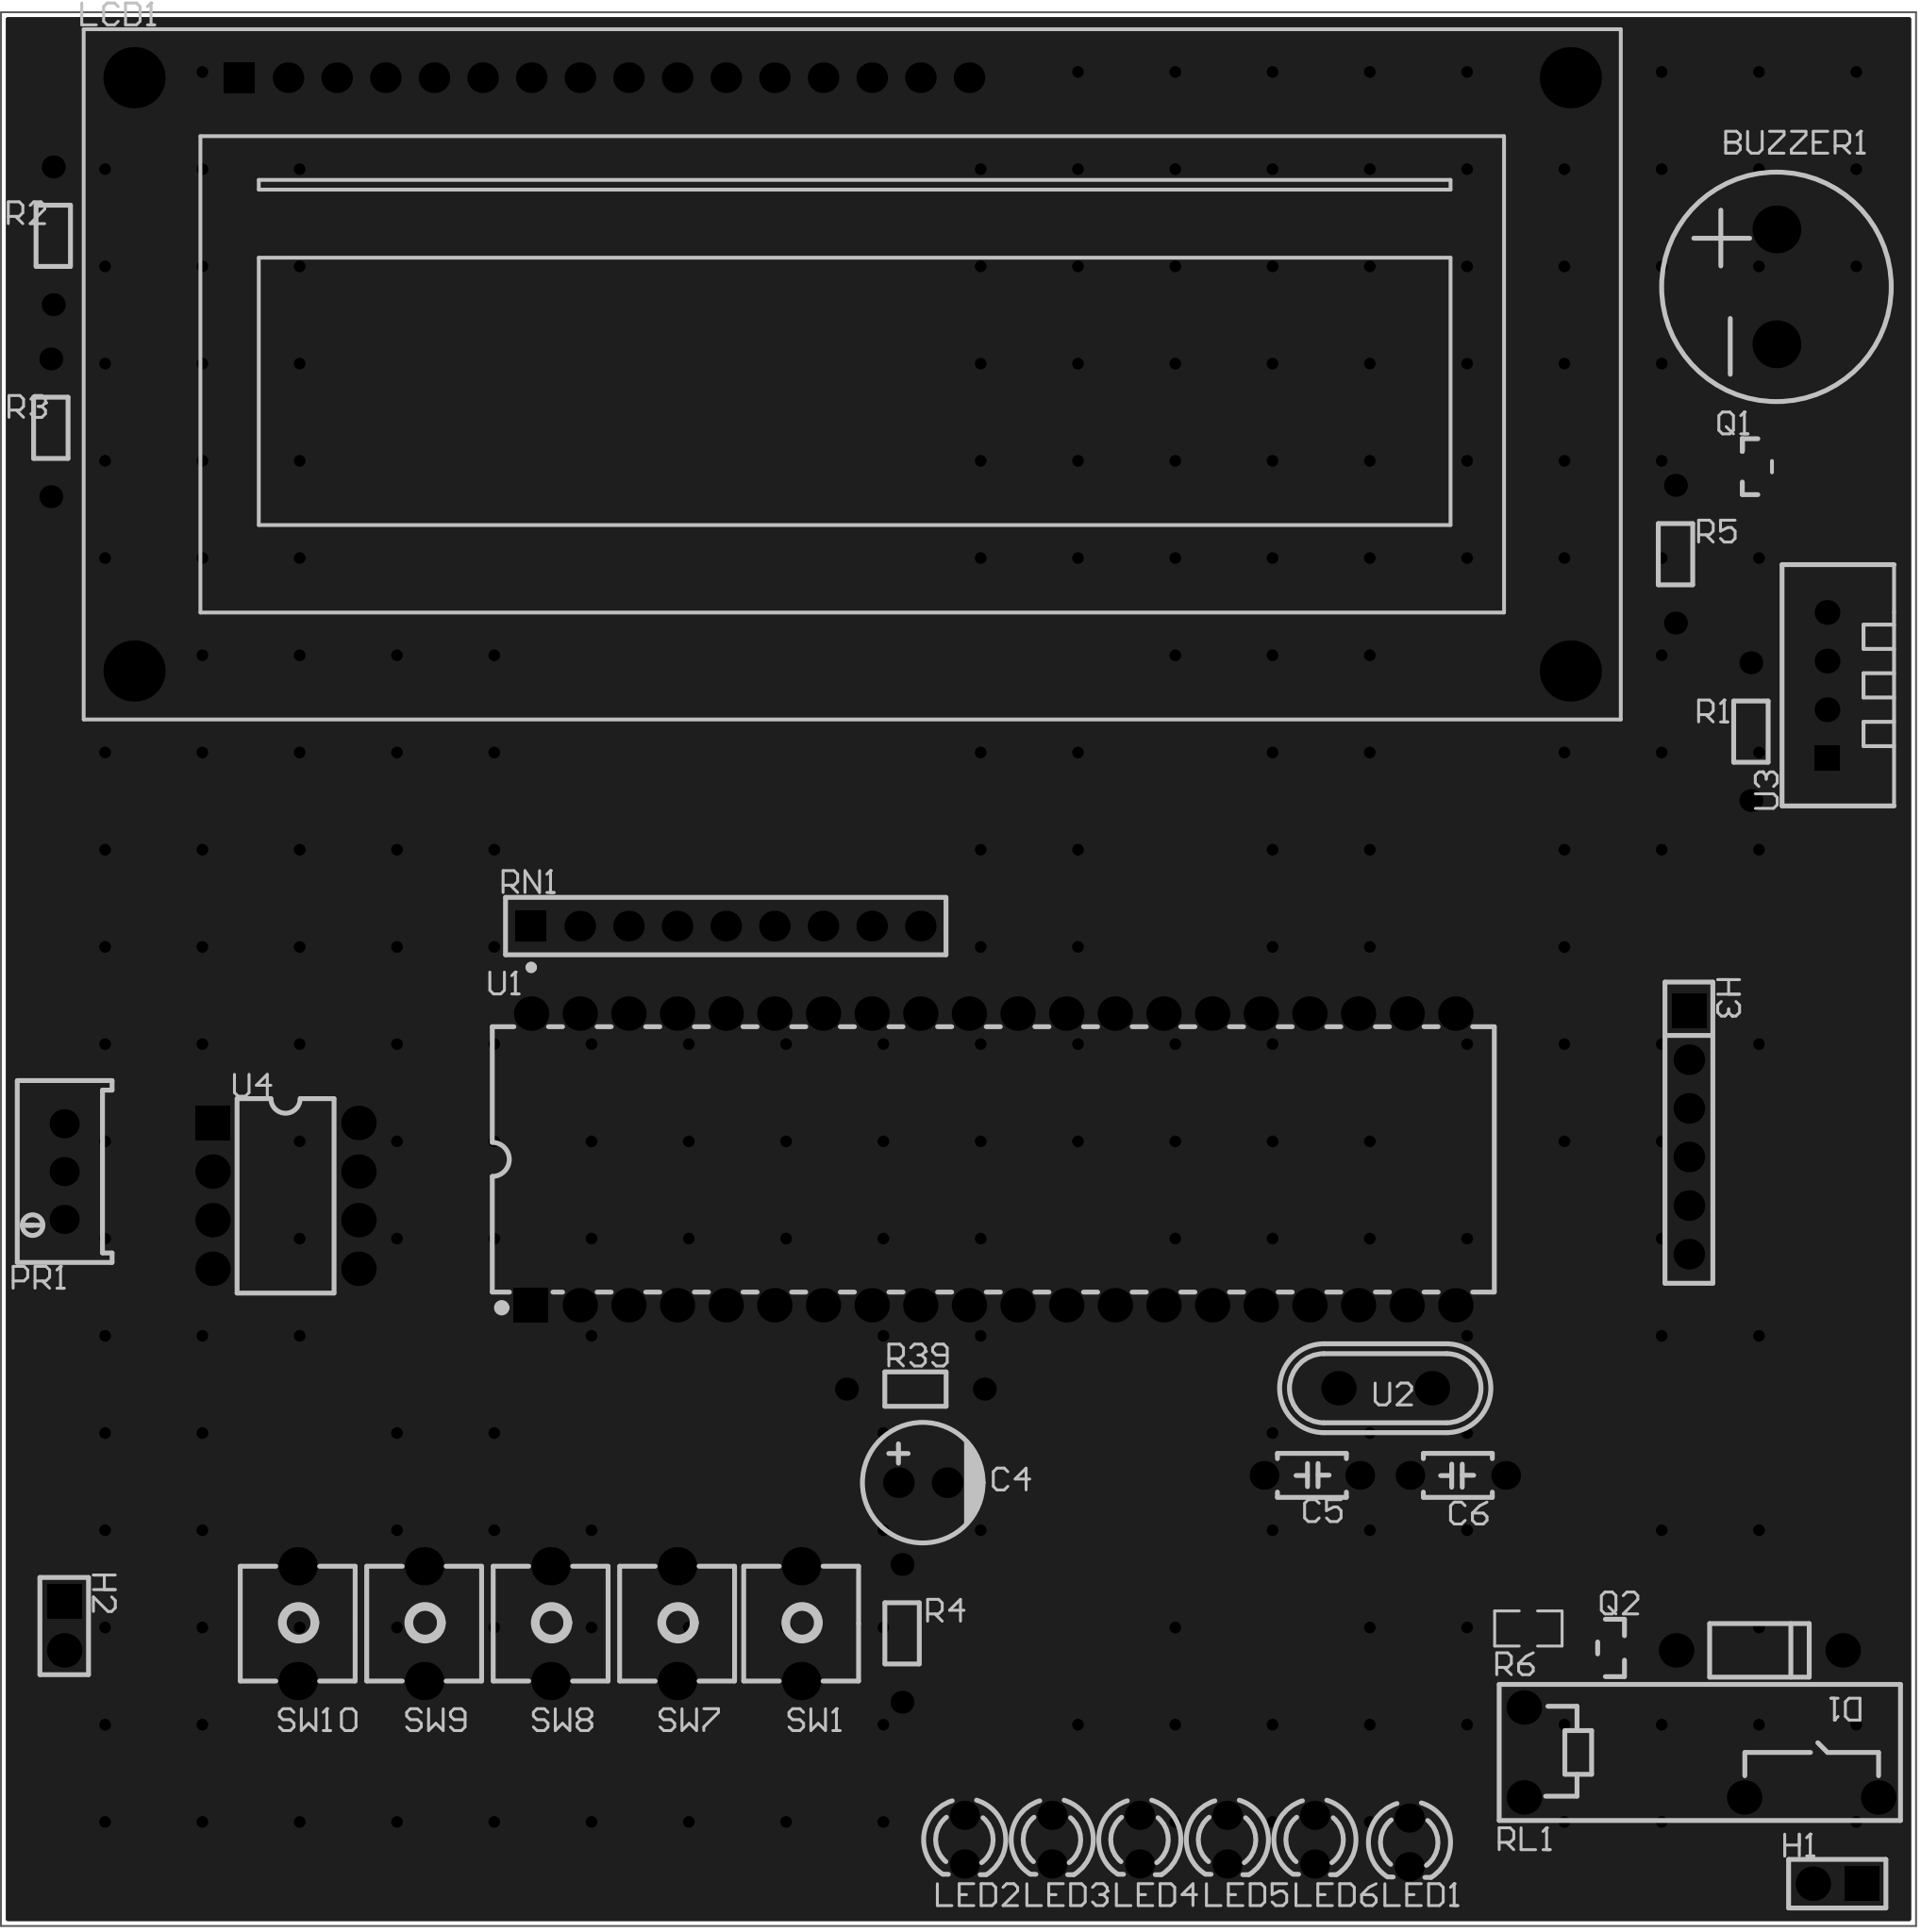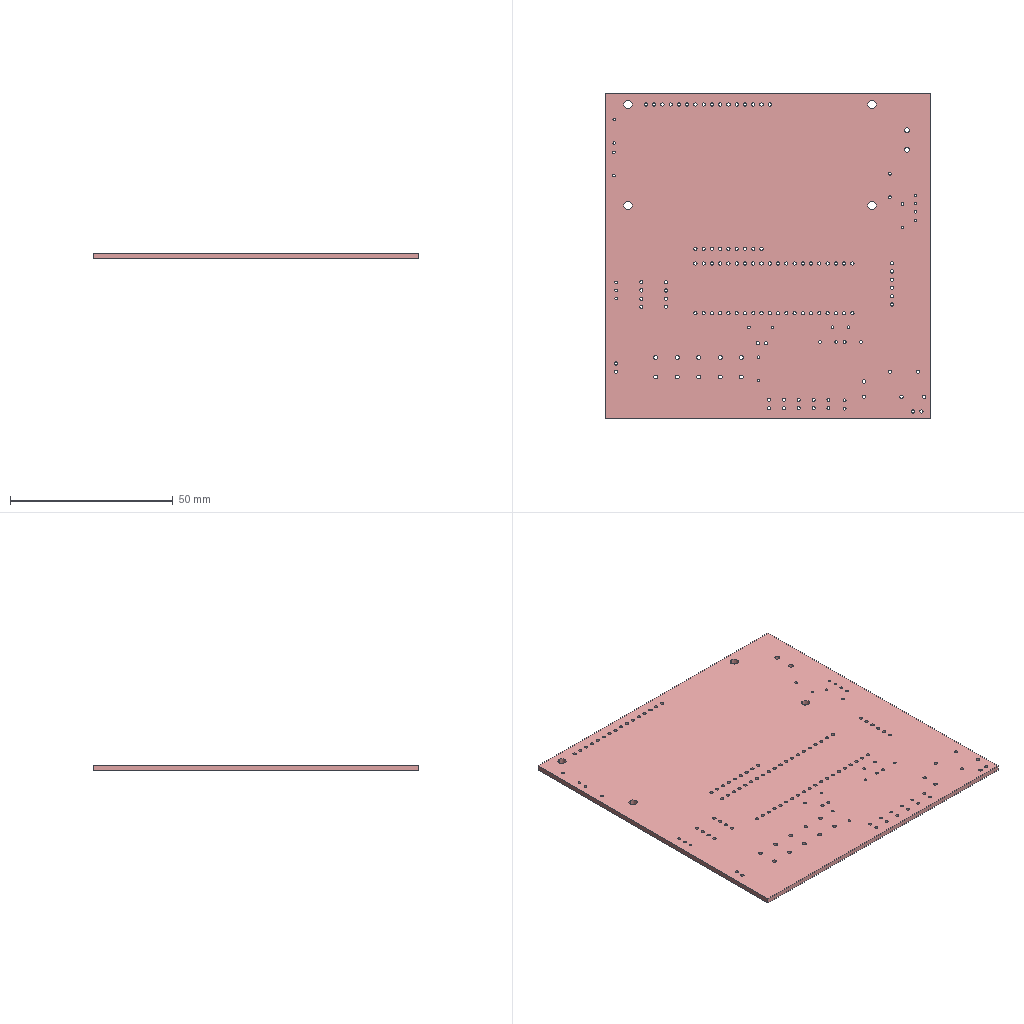Circuit board layout | Altium Designer | box 100 x 100 x 1.6 mm
Layer stack:
# Altium Designer layer stack of  (unit mm; dielectric type: 0 none, 1 core, 2 prepreg, 3 surface material)
index,name,kind,layer,copper_thickness_mm,dielectric_type,dielectric_thickness_mm,dielectric_material,dielectric_constant
0,Top Paste Mask Layer,other,,,,,,
1,Top Silkscreen Layer,other,,,,,,
2,Top Solder Mask Layer,dielectric,,,3,0.01,,3.3
3,Top Layer,copper,Top Layer,0.035,,,,
4,Dielectric1,dielectric,,,3,1.51,FR4,4.5
5,Bottom Layer,copper,Bottom Layer,0.035,,,,
6,Bottom Solder Mask Layer,dielectric,,,3,0.01,,3.3
7,Bottom Silkscreen Layer,other,,,,,,
8,Bottom Paste Mask Layer,other,,,,,,
# drill layer pairs: low layer,high layer
drill_pair,Top Layer,Bottom Layer
Part placement:
Designator,Comment,Layer,Footprint,Center-X(mm),Center-Y(mm),Rotation
C4,10uF,TopLayer,CAP-TH_BD6.3-P2.50-D1.0-FD,133.096,111.76,0
U1,STC89C52,TopLayer,DIP-40_L52.3-W13.9-P2.54-LS15.2-BL,136.779,128.651,0
U2,12MHz,TopLayer,HC-49US_L11.0-W4.6-P4.88,157.244,116.695,0
C5,30pF,TopLayer,CAP-TH_L3.6-W2.3-P5.00-D0.5,153.416,112.141,0
C6,30pF,TopLayer,CAP-TH_L3.6-W2.3-P5.00-D0.5,161.036,112.141,180
R39,10kΩ,TopLayer,Res_1/8W,132.715,116.649,0
SW7,Tact switch, 6*6*5 plastic head, 260G, travel 0.25mm, through-hole 2-pin,TopLayer,KEY-TH_2P-L6.0-W6.0-P5.00,120.269,104.394,90
SW8,Tact switch, 6*6*5 plastic head, 260G, travel 0.25mm, through-hole 2-pin,TopLayer,KEY-TH_2P-L6.0-W6.0-P5.00,113.665,104.394,90
SW9,Tact switch, 6*6*5 plastic head, 260G, travel 0.25mm, through-hole 2-pin,TopLayer,KEY-TH_2P-L6.0-W6.0-P5.00,107.061,104.394,90
SW10,Tact switch, 6*6*5 plastic head, 260G, travel 0.25mm, through-hole 2-pin,TopLayer,KEY-TH_2P-L6.0-W6.0-P5.00,100.457,104.394,90
BUZZER1,buzzer,TopLayer,BUZ-TH_BD12.0-P6.00-D0.9-RD,177.673,174.244,90
D1,,TopLayer,DO_1N4007,176.784,102.997,180
H1,,TopLayer,HDR-TH_2P-P2.54-V-M-1,180.848,90.805,180
LCD1,HS1602A,TopLayer,LCD1602,129.413,169.672,0
LED3,,TopLayer,LED_TH-3mm,139.842,93.106,270
LED4,,TopLayer,LED_TH-3mm,144.414,93.106,270
LED5,,TopLayer,LED_TH-3mm,148.986,93.106,270
LED6,,TopLayer,LED_TH-3mm,153.558,93.106,270
PR1,10kΩ,TopLayer,R_3296,88.265,128.016,90
Q1,,TopLayer,S8550P_SOT,176.54,164.847,0
Q2,,TopLayer,S8050_SOT-23,169.037,103.124,180
R1,10kΩ,TopLayer,Res_1/8W,176.339,151.003,270
R4,10kΩ,TopLayer,Res_1/8W,132.016,103.886,270
R5,2.2kΩ,TopLayer,Res_1/8W,172.402,160.274,270
R6,1K,TopLayer,R0805,164.719,104.14,180
RL1,HT46F-DC12V-SHAG,TopLayer,RELAY-TH_HT46F-DCXXV-SHAG,173.736,97.663,0
RN1,-,TopLayer,RES-ARRAY-TH_9P-P2.54-D1.0,122.809,140.843,0
SW1,Tact switch, 6*6*5 plastic head, 260G, travel 0.25mm, through-hole 2-pin,TopLayer,KEY-TH_2P-L6.0-W6.0-P5.00,126.746,104.394,90
LED1,,TopLayer,LED_TH-3mm,158.496,92.964,270
LED2,,TopLayer,LED_TH-3mm,135.27,93.106,270
U3,DHT11,TopLayer,SENSOR-TH_DHT11,180.314,153.42,90
U4,ADC0832CCN,TopLayer,DIP-8_L9.7-W6.4-P2.54-LS7.6-BL,99.822,126.746,270
R2,10kΩ,TopLayer,Res_1/8W,87.694,176.911,90
R3,1kΩ,TopLayer,Res_1/8W,87.567,166.878,90
H2,,TopLayer,HDR-TH_2P-P2.54-V-M-1,88.265,104.267,270
H3,,TopLayer,HDR-TH_6P-P2.54-V-F,173.101,130.048,270
Pad and via stacks:
# Altium Designer via and pad stacks of  (unit mm). Each distinct definition once, with the count of objects using it.
# via: kind,start_layer,end_layer,hole_mm,diameter_mm,mode(0 simple;1 top-mid-bottom;2 full stack),diameter_per_layer,count,example_net
# pad: kind,layer,hole_mm,hole_type(0 round;1 square;2 slot),plating,top_size,top_shape(1 round;2 rect;3 octagon;9 rounded rect),mid_size,bottom_size,mode,footprint,size_per_layer,count,example
pad,Multi-Layer,1,0,plated,1.6x1.6,1,1.6x1.6,1.6x1.6,0,CAP-TH_BD6.3-P2.50-D1.0-FD,,2,C4.1
pad,Multi-Layer,1,0,plated,1.8x1.8,1,1.8x1.8,1.8x1.8,0,DIP-40_L52.3-W13.9-P2.54-LS15.2-BL,,39,U1.19
pad,Multi-Layer,1,0,plated,1.8x1.8,2,1.8x1.8,1.8x1.8,0,DIP-40_L52.3-W13.9-P2.54-LS15.2-BL,,1,U1.1
pad,Multi-Layer,0.8,0,plated,1.8x1.8,1,1.8x1.8,1.8x1.8,0,HC-49US_L11.0-W4.6-P4.88,,2,U2.1
pad,Multi-Layer,0.9,0,plated,1.5x1.5,1,1.5x1.5,1.5x1.5,0,CAP-TH_L3.6-W2.3-P5.00-D0.5,,4,C5.1
pad,Multi-Layer,0.8001,0,plated,1.199x1.199,1,1.199x1.199,1.199x1.199,0,Res_1/8W,,12,R39.1
pad,Multi-Layer,1.2,0,plated,2x2,1,2x2,2x2,0,KEY-TH_2P-L6.0-W6.0-P5.00,,10,SW7.2
pad,Multi-Layer,1.5,0,plated,2.5x2.5,1,2.5x2.5,2.5x2.5,0,BUZ-TH_BD12.0-P6.00-D0.9-RD,,2,BUZZER1.1
pad,Multi-Layer,1,0,plated,1.8x1.8,1,1.8x1.8,1.8x1.8,0,DO_1N4007,,2,D1.1
pad,Multi-Layer,1,0,plated,1.8x1.8,1,1.8x1.8,1.8x1.8,0,HDR-TH_2P-P2.54-V-M-1,,2,H1.2
pad,Multi-Layer,1,0,plated,1.8x1.8,2,1.8x1.8,1.8x1.8,0,HDR-TH_2P-P2.54-V-M-1,,2,H1.1
pad,Multi-Layer,1,0,plated,1.6x1.6,1,1.6x1.6,1.6x1.6,0,LCD1602,,15,LCD1.16
pad,Multi-Layer,1,0,plated,1.6x1.6,2,1.6x1.6,1.6x1.6,0,LCD1602,,1,LCD1.1
pad,Multi-Layer,2.5,2,plated,3.2x3.2,1,3.2x3.2,3.2x3.2,0,LCD1602,,4,LCD1.0
pad,Multi-Layer,0.9144,0,plated,1.524x1.524,1,1.524x1.524,1.524x1.524,0,LED_TH-3mm,,12,LED3.1
pad,Multi-Layer,0.762,0,plated,1.524x1.524,1,1.524x1.524,1.524x1.524,0,R_3296,,3,PR1.2
pad,Multi-Layer,1.1,0,plated,1.8x1.8,1,1.8x1.8,1.8x1.8,0,RELAY-TH_HT46F-DCXXV-SHAG,,4,RL1.1
pad,Multi-Layer,1,0,plated,1.6x1.6,2,1.6x1.6,1.6x1.6,0,RES-ARRAY-TH_9P-P2.54-D1.0,,1,RN1.1
pad,Multi-Layer,1,0,plated,1.6x1.6,1,1.6x1.6,1.6x1.6,0,RES-ARRAY-TH_9P-P2.54-D1.0,,8,RN1.2
pad,Multi-Layer,0.7112,0,plated,1.295x1.295,2,1.295x1.295,1.295x1.295,0,SENSOR-TH_DHT11,,1,U3.1
pad,Multi-Layer,0.7112,0,plated,1.295x1.295,1,1.295x1.295,1.295x1.295,0,SENSOR-TH_DHT11,,3,U3.2
pad,Multi-Layer,1,0,plated,1.8x1.8,2,1.8x1.8,1.8x1.8,0,DIP-8_L9.7-W6.4-P2.54-LS7.6-BL,,1,U4.1
pad,Multi-Layer,1,0,plated,1.8x1.8,1,1.8x1.8,1.8x1.8,0,DIP-8_L9.7-W6.4-P2.54-LS7.6-BL,,7,U4.2
pad,Multi-Layer,1.02,0,plated,1.6x1.6,1,1.6x1.6,1.6x1.6,0,HDR-TH_6P-P2.54-V-F,,5,H3.6
pad,Multi-Layer,1.02,0,plated,1.8x1.8,2,1.8x1.8,1.8x1.8,0,HDR-TH_6P-P2.54-V-F,,1,H3.1
pad,Top Layer,0,0,plated,0.701x1.25,2,0.701x1.25,0.701x1.25,0,S8550P_SOT,,3,Q1.3
pad,Top Layer,0,0,plated,1x0.8,2,1x0.8,1x0.8,0,S8050_SOT-23,,3,Q2.2
pad,Top Layer,0,0,plated,1.133x1.377,2,1.133x1.377,1.133x1.377,0,R0805,,2,R6.2
via,Top Layer,Bottom Layer,0.3048,0.61,0,,226,GND
Copper pours:
name,layer,net,type(0 solid;1 hatched;2 none)
Bottom Layer-GND,Bottom Layer,GND,0
Top Layer-GND,Top Layer,GND,0